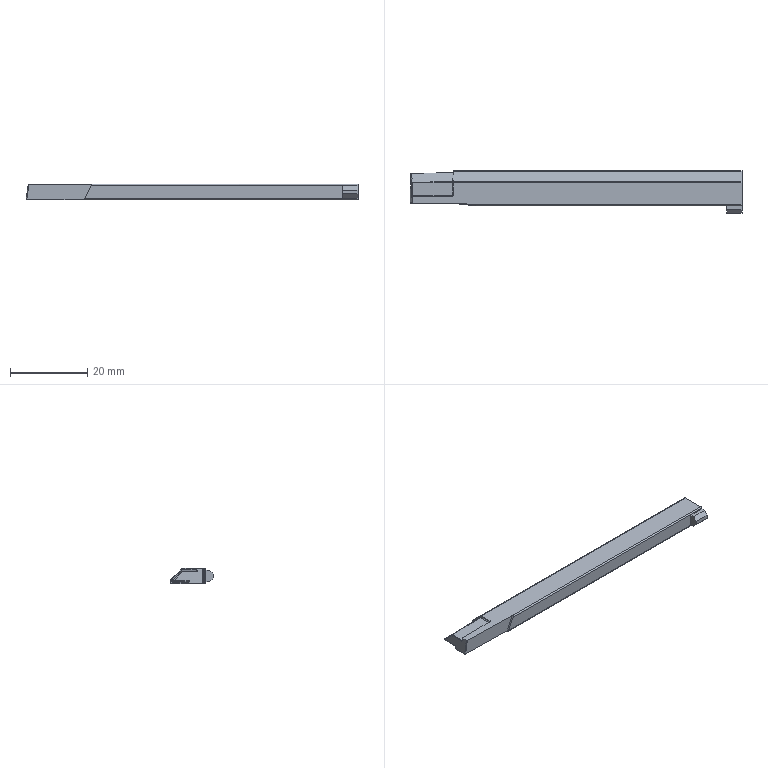Part | Creo | 1 solid | 55 faces | box 85.892 x 11.1 x 4 mm | volume 2633 mm3 | cylinder 22 | plane 21 | spline 6 | sphere 5 | torus 1 | commonest cylinder face diameters 0.402 x17 0.6 x2 1 x2 2 x1